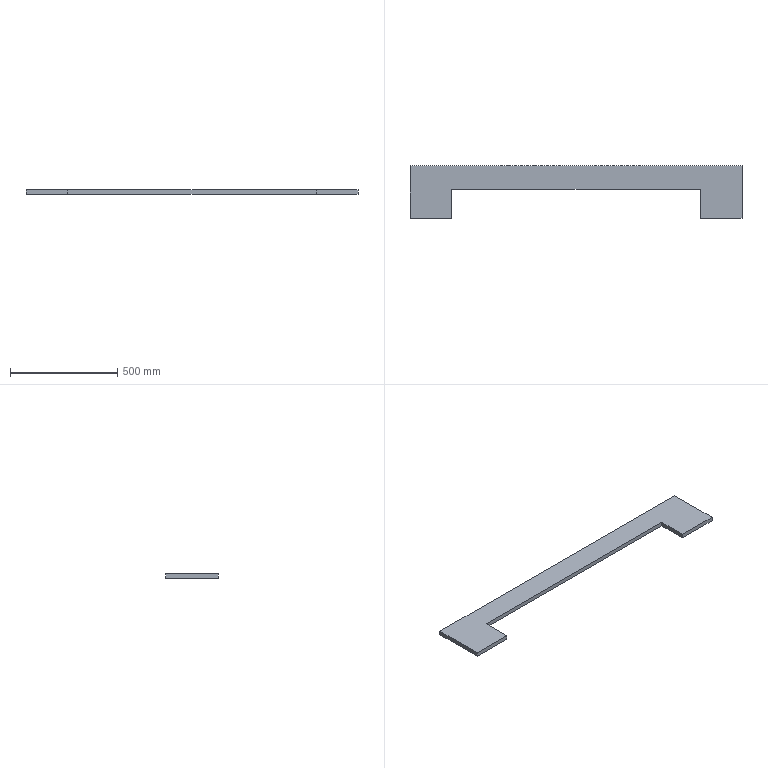Part | SolidWorks | features BaseBody 1 | 1 solid | 10 faces | box 1550 x 247 x 20 mm | volume 4478600 mm3 | plane 10
STEP:
#1=CARTESIAN_POINT('',(775.,-122.,20.));
#2=VERTEX_POINT('',#1);
#3=CARTESIAN_POINT('',(580.,-122.,20.));
#4=VERTEX_POINT('',#3);
#5=CARTESIAN_POINT('',(580.,-122.,20.));
#6=DIRECTION('',(-1.,0.,0.));
#7=VECTOR('',#6,1000.);
#8=LINE('',#5,#7);
#9=EDGE_CURVE('',#2,#4,#8,.T.);
#10=ORIENTED_EDGE('',*,*,#9,.F.);
#11=CARTESIAN_POINT('',(775.,125.,20.));
#12=VERTEX_POINT('',#11);
#13=CARTESIAN_POINT('',(775.,125.,20.));
#14=DIRECTION('',(0.,1.,0.));
#15=VECTOR('',#14,1000.);
#16=LINE('',#13,#15);
#17=EDGE_CURVE('',#2,#12,#16,.T.);
#18=ORIENTED_EDGE('',*,*,#17,.T.);
#19=CARTESIAN_POINT('',(-775.,125.,20.));
#20=VERTEX_POINT('',#19);
#21=CARTESIAN_POINT('',(-775.,125.,20.));
#22=DIRECTION('',(-1.,0.,0.));
#23=VECTOR('',#22,1000.);
#24=LINE('',#21,#23);
#25=EDGE_CURVE('',#12,#20,#24,.T.);
#26=ORIENTED_EDGE('',*,*,#25,.T.);
#27=CARTESIAN_POINT('',(-775.,-122.,20.));
#28=VERTEX_POINT('',#27);
#29=CARTESIAN_POINT('',(-775.,125.,20.));
#30=DIRECTION('',(0.,-1.,0.));
#31=VECTOR('',#30,1000.);
#32=LINE('',#29,#31);
#33=EDGE_CURVE('',#20,#28,#32,.T.);
#34=ORIENTED_EDGE('',*,*,#33,.T.);
#35=CARTESIAN_POINT('',(-580.,-122.,20.));
#36=VERTEX_POINT('',#35);
#37=CARTESIAN_POINT('',(-775.,-122.,20.));
#38=DIRECTION('',(-1.,0.,0.));
#39=VECTOR('',#38,1000.);
#40=LINE('',#37,#39);
#41=EDGE_CURVE('',#36,#28,#40,.T.);
#42=ORIENTED_EDGE('',*,*,#41,.F.);
#43=CARTESIAN_POINT('',(-580.,15.,20.));
#44=VERTEX_POINT('',#43);
#45=CARTESIAN_POINT('',(-580.,15.,20.));
#46=DIRECTION('',(0.,1.,0.));
#47=VECTOR('',#46,1000.);
#48=LINE('',#45,#47);
#49=EDGE_CURVE('',#36,#44,#48,.T.);
#50=ORIENTED_EDGE('',*,*,#49,.T.);
#51=CARTESIAN_POINT('',(580.,15.,20.));
#52=VERTEX_POINT('',#51);
#53=CARTESIAN_POINT('',(-580.,15.,20.));
#54=DIRECTION('',(1.,0.,0.));
#55=VECTOR('',#54,1000.);
#56=LINE('',#53,#55);
#57=EDGE_CURVE('',#44,#52,#56,.T.);
#58=ORIENTED_EDGE('',*,*,#57,.T.);
#59=CARTESIAN_POINT('',(580.,15.,20.));
#60=DIRECTION('',(0.,-1.,0.));
#61=VECTOR('',#60,1000.);
#62=LINE('',#59,#61);
#63=EDGE_CURVE('',#52,#4,#62,.T.);
#64=ORIENTED_EDGE('',*,*,#63,.T.);
#65=EDGE_LOOP('',(#10,#18,#26,#34,#42,#50,#58,#64));
#66=FACE_OUTER_BOUND('',#65,.T.);
#67=CARTESIAN_POINT('',(0.,0.,20.));
#68=DIRECTION('',(0.,0.,-1.));
#69=DIRECTION('',(-1.,0.,0.));
#70=AXIS2_PLACEMENT_3D('',#67,#68,#69);
#71=PLANE('',#70);
#72=ADVANCED_FACE('',(#66),#71,.F.);
#73=CARTESIAN_POINT('',(775.,-122.,0.));
#74=VERTEX_POINT('',#73);
#75=CARTESIAN_POINT('',(775.,125.,0.));
#76=VERTEX_POINT('',#75);
#77=CARTESIAN_POINT('',(775.,125.,0.));
#78=DIRECTION('',(0.,1.,0.));
#79=VECTOR('',#78,1000.);
#80=LINE('',#77,#79);
#81=EDGE_CURVE('',#74,#76,#80,.T.);
#82=ORIENTED_EDGE('',*,*,#81,.F.);
#83=CARTESIAN_POINT('',(580.,-122.,0.));
#84=VERTEX_POINT('',#83);
#85=CARTESIAN_POINT('',(0.,-122.,0.));
#86=DIRECTION('',(-1.,0.,0.));
#87=VECTOR('',#86,1000.);
#88=LINE('',#85,#87);
#89=EDGE_CURVE('',#74,#84,#88,.T.);
#90=ORIENTED_EDGE('',*,*,#89,.T.);
#91=CARTESIAN_POINT('',(580.,15.,0.));
#92=VERTEX_POINT('',#91);
#93=CARTESIAN_POINT('',(580.,15.,0.));
#94=DIRECTION('',(0.,-1.,0.));
#95=VECTOR('',#94,1000.);
#96=LINE('',#93,#95);
#97=EDGE_CURVE('',#92,#84,#96,.T.);
#98=ORIENTED_EDGE('',*,*,#97,.F.);
#99=CARTESIAN_POINT('',(-580.,15.,0.));
#100=VERTEX_POINT('',#99);
#101=CARTESIAN_POINT('',(-580.,15.,0.));
#102=DIRECTION('',(1.,0.,0.));
#103=VECTOR('',#102,1000.);
#104=LINE('',#101,#103);
#105=EDGE_CURVE('',#100,#92,#104,.T.);
#106=ORIENTED_EDGE('',*,*,#105,.F.);
#107=CARTESIAN_POINT('',(-580.,-122.,0.));
#108=VERTEX_POINT('',#107);
#109=CARTESIAN_POINT('',(-580.,15.,0.));
#110=DIRECTION('',(0.,1.,0.));
#111=VECTOR('',#110,1000.);
#112=LINE('',#109,#111);
#113=EDGE_CURVE('',#108,#100,#112,.T.);
#114=ORIENTED_EDGE('',*,*,#113,.F.);
#115=CARTESIAN_POINT('',(-775.,-122.,0.));
#116=VERTEX_POINT('',#115);
#117=CARTESIAN_POINT('',(0.,-122.,0.));
#118=DIRECTION('',(-1.,0.,0.));
#119=VECTOR('',#118,1000.);
#120=LINE('',#117,#119);
#121=EDGE_CURVE('',#108,#116,#120,.T.);
#122=ORIENTED_EDGE('',*,*,#121,.T.);
#123=CARTESIAN_POINT('',(-775.,125.,0.));
#124=VERTEX_POINT('',#123);
#125=CARTESIAN_POINT('',(-775.,125.,0.));
#126=DIRECTION('',(0.,-1.,0.));
#127=VECTOR('',#126,1000.);
#128=LINE('',#125,#127);
#129=EDGE_CURVE('',#124,#116,#128,.T.);
#130=ORIENTED_EDGE('',*,*,#129,.F.);
#131=CARTESIAN_POINT('',(-775.,125.,0.));
#132=DIRECTION('',(-1.,0.,0.));
#133=VECTOR('',#132,1000.);
#134=LINE('',#131,#133);
#135=EDGE_CURVE('',#76,#124,#134,.T.);
#136=ORIENTED_EDGE('',*,*,#135,.F.);
#137=EDGE_LOOP('',(#82,#90,#98,#106,#114,#122,#130,#136));
#138=FACE_OUTER_BOUND('',#137,.T.);
#139=CARTESIAN_POINT('',(0.,0.,0.));
#140=DIRECTION('',(0.,0.,-1.));
#141=DIRECTION('',(-1.,0.,0.));
#142=AXIS2_PLACEMENT_3D('',#139,#140,#141);
#143=PLANE('',#142);
#144=ADVANCED_FACE('',(#138),#143,.T.);
#145=CARTESIAN_POINT('',(775.,-122.,20.));
#146=DIRECTION('',(0.,0.,1.));
#147=VECTOR('',#146,1000.);
#148=LINE('',#145,#147);
#149=EDGE_CURVE('',#74,#2,#148,.T.);
#150=ORIENTED_EDGE('',*,*,#149,.F.);
#151=ORIENTED_EDGE('',*,*,#81,.T.);
#152=CARTESIAN_POINT('',(775.,125.,20.));
#153=DIRECTION('',(0.,0.,-1.));
#154=VECTOR('',#153,1000.);
#155=LINE('',#152,#154);
#156=EDGE_CURVE('',#12,#76,#155,.T.);
#157=ORIENTED_EDGE('',*,*,#156,.F.);
#158=ORIENTED_EDGE('',*,*,#17,.F.);
#159=EDGE_LOOP('',(#150,#151,#157,#158));
#160=FACE_OUTER_BOUND('',#159,.T.);
#161=CARTESIAN_POINT('',(775.,125.,20.));
#162=DIRECTION('',(-1.,0.,0.));
#163=DIRECTION('',(0.,0.,1.));
#164=AXIS2_PLACEMENT_3D('',#161,#162,#163);
#165=PLANE('',#164);
#166=ADVANCED_FACE('',(#160),#165,.F.);
#167=CARTESIAN_POINT('',(580.,-122.,20.));
#168=DIRECTION('',(0.,0.,-1.));
#169=VECTOR('',#168,1000.);
#170=LINE('',#167,#169);
#171=EDGE_CURVE('',#4,#84,#170,.T.);
#172=ORIENTED_EDGE('',*,*,#171,.F.);
#173=ORIENTED_EDGE('',*,*,#63,.F.);
#174=CARTESIAN_POINT('',(580.,15.,20.));
#175=DIRECTION('',(0.,0.,-1.));
#176=VECTOR('',#175,1000.);
#177=LINE('',#174,#176);
#178=EDGE_CURVE('',#52,#92,#177,.T.);
#179=ORIENTED_EDGE('',*,*,#178,.T.);
#180=ORIENTED_EDGE('',*,*,#97,.T.);
#181=EDGE_LOOP('',(#172,#173,#179,#180));
#182=FACE_OUTER_BOUND('',#181,.T.);
#183=CARTESIAN_POINT('',(580.,15.,20.));
#184=DIRECTION('',(1.,0.,0.));
#185=DIRECTION('',(0.,0.,-1.));
#186=AXIS2_PLACEMENT_3D('',#183,#184,#185);
#187=PLANE('',#186);
#188=ADVANCED_FACE('',(#182),#187,.F.);
#189=CARTESIAN_POINT('',(-775.,-122.,20.));
#190=DIRECTION('',(0.,0.,-1.));
#191=VECTOR('',#190,1000.);
#192=LINE('',#189,#191);
#193=EDGE_CURVE('',#28,#116,#192,.T.);
#194=ORIENTED_EDGE('',*,*,#193,.F.);
#195=ORIENTED_EDGE('',*,*,#33,.F.);
#196=CARTESIAN_POINT('',(-775.,125.,20.));
#197=DIRECTION('',(0.,0.,-1.));
#198=VECTOR('',#197,1000.);
#199=LINE('',#196,#198);
#200=EDGE_CURVE('',#20,#124,#199,.T.);
#201=ORIENTED_EDGE('',*,*,#200,.T.);
#202=ORIENTED_EDGE('',*,*,#129,.T.);
#203=EDGE_LOOP('',(#194,#195,#201,#202));
#204=FACE_OUTER_BOUND('',#203,.T.);
#205=CARTESIAN_POINT('',(-775.,125.,20.));
#206=DIRECTION('',(1.,0.,0.));
#207=DIRECTION('',(0.,0.,-1.));
#208=AXIS2_PLACEMENT_3D('',#205,#206,#207);
#209=PLANE('',#208);
#210=ADVANCED_FACE('',(#204),#209,.F.);
#211=CARTESIAN_POINT('',(-580.,-122.,20.));
#212=DIRECTION('',(0.,0.,1.));
#213=VECTOR('',#212,1000.);
#214=LINE('',#211,#213);
#215=EDGE_CURVE('',#108,#36,#214,.T.);
#216=ORIENTED_EDGE('',*,*,#215,.F.);
#217=ORIENTED_EDGE('',*,*,#113,.T.);
#218=CARTESIAN_POINT('',(-580.,15.,20.));
#219=DIRECTION('',(0.,0.,-1.));
#220=VECTOR('',#219,1000.);
#221=LINE('',#218,#220);
#222=EDGE_CURVE('',#44,#100,#221,.T.);
#223=ORIENTED_EDGE('',*,*,#222,.F.);
#224=ORIENTED_EDGE('',*,*,#49,.F.);
#225=EDGE_LOOP('',(#216,#217,#223,#224));
#226=FACE_OUTER_BOUND('',#225,.T.);
#227=CARTESIAN_POINT('',(-580.,15.,20.));
#228=DIRECTION('',(-1.,0.,0.));
#229=DIRECTION('',(0.,0.,1.));
#230=AXIS2_PLACEMENT_3D('',#227,#228,#229);
#231=PLANE('',#230);
#232=ADVANCED_FACE('',(#226),#231,.F.);
#233=ORIENTED_EDGE('',*,*,#135,.T.);
#234=ORIENTED_EDGE('',*,*,#200,.F.);
#235=ORIENTED_EDGE('',*,*,#25,.F.);
#236=ORIENTED_EDGE('',*,*,#156,.T.);
#237=EDGE_LOOP('',(#233,#234,#235,#236));
#238=FACE_OUTER_BOUND('',#237,.T.);
#239=CARTESIAN_POINT('',(-775.,125.,20.));
#240=DIRECTION('',(0.,-1.,0.));
#241=DIRECTION('',(0.,0.,-1.));
#242=AXIS2_PLACEMENT_3D('',#239,#240,#241);
#243=PLANE('',#242);
#244=ADVANCED_FACE('',(#238),#243,.F.);
#245=ORIENTED_EDGE('',*,*,#105,.T.);
#246=ORIENTED_EDGE('',*,*,#178,.F.);
#247=ORIENTED_EDGE('',*,*,#57,.F.);
#248=ORIENTED_EDGE('',*,*,#222,.T.);
#249=EDGE_LOOP('',(#245,#246,#247,#248));
#250=FACE_OUTER_BOUND('',#249,.T.);
#251=CARTESIAN_POINT('',(-580.,15.,20.));
#252=DIRECTION('',(0.,1.,0.));
#253=DIRECTION('',(0.,0.,1.));
#254=AXIS2_PLACEMENT_3D('',#251,#252,#253);
#255=PLANE('',#254);
#256=ADVANCED_FACE('',(#250),#255,.F.);
#257=ORIENTED_EDGE('',*,*,#215,.T.);
#258=ORIENTED_EDGE('',*,*,#41,.T.);
#259=ORIENTED_EDGE('',*,*,#193,.T.);
#260=ORIENTED_EDGE('',*,*,#121,.F.);
#261=EDGE_LOOP('',(#257,#258,#259,#260));
#262=FACE_OUTER_BOUND('',#261,.T.);
#263=CARTESIAN_POINT('',(0.,-122.,-65.));
#264=DIRECTION('',(0.,-1.,0.));
#265=DIRECTION('',(0.,0.,-1.));
#266=AXIS2_PLACEMENT_3D('',#263,#264,#265);
#267=PLANE('',#266);
#268=ADVANCED_FACE('',(#262),#267,.T.);
#269=ORIENTED_EDGE('',*,*,#149,.T.);
#270=ORIENTED_EDGE('',*,*,#9,.T.);
#271=ORIENTED_EDGE('',*,*,#171,.T.);
#272=ORIENTED_EDGE('',*,*,#89,.F.);
#273=EDGE_LOOP('',(#269,#270,#271,#272));
#274=FACE_OUTER_BOUND('',#273,.T.);
#275=CARTESIAN_POINT('',(0.,-122.,-65.));
#276=DIRECTION('',(0.,-1.,0.));
#277=DIRECTION('',(0.,0.,-1.));
#278=AXIS2_PLACEMENT_3D('',#275,#276,#277);
#279=PLANE('',#278);
#280=ADVANCED_FACE('',(#274),#279,.T.);
#281=CLOSED_SHELL('',(#72,#144,#166,#188,#210,#232,#244,#256,#268,#280));
#282=MANIFOLD_SOLID_BREP('',#281);
#283=CARTESIAN_POINT('',(0.,0.,0.));
#284=DIRECTION('',(0.,0.,1.));
#285=DIRECTION('',(1.,0.,0.));
#286=AXIS2_PLACEMENT_3D('',#283,#284,#285);
#287=(LENGTH_UNIT()NAMED_UNIT(*)SI_UNIT(.MILLI.,.METRE.));
#288=UNCERTAINTY_MEASURE_WITH_UNIT(LENGTH_MEASURE(0.00001),#287,'','');
#289=(NAMED_UNIT(*)PLANE_ANGLE_UNIT()SI_UNIT($,.RADIAN.));
#290=(NAMED_UNIT(*)SI_UNIT($,.STERADIAN.)SOLID_ANGLE_UNIT());
#291=(GEOMETRIC_REPRESENTATION_CONTEXT(3)GLOBAL_UNCERTAINTY_ASSIGNED_CONTEXT((#288))GLOBAL_UNIT_ASSIGNED_CONTEXT((#287,#289,#290))REPRESENTATION_CONTEXT('',''));
#292=ADVANCED_BREP_SHAPE_REPRESENTATION('',(#282,#286),#291);